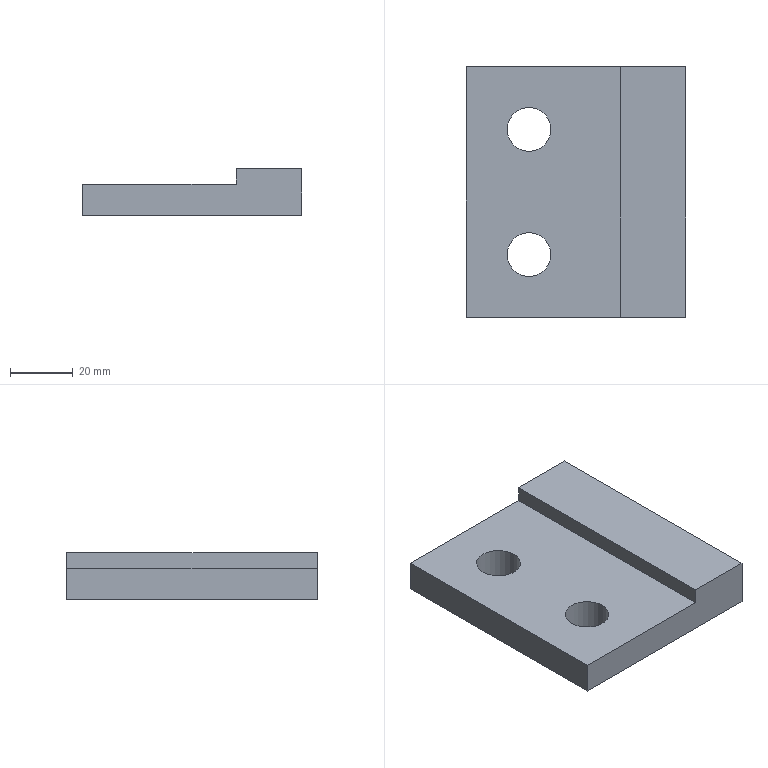Part | NX | features solid 2 | 1 solid | 10 faces | box 70 x 80 x 15 mm | volume 61270 mm3 | plane 8 | cylinder 2 | commonest cylinder face diameters 14 x2
STEP:
#1=CARTESIAN_POINT('',(18.,860.,-27.021));
#2=VERTEX_POINT('',#1);
#3=CARTESIAN_POINT('',(25.,860.,-27.021));
#4=DIRECTION('',(0.,0.,1.));
#5=DIRECTION('',(-1.,0.,0.));
#6=AXIS2_PLACEMENT_3D('',#3,#4,#5);
#7=CIRCLE('',#6,7.);
#8=EDGE_CURVE('',#2,#2,#7,.F.);
#9=ORIENTED_EDGE('',*,*,#8,.T.);
#10=EDGE_LOOP('',(#9));
#11=FACE_BOUND('',#10,.T.);
#12=CARTESIAN_POINT('',(54.128,880.,-27.021));
#13=VERTEX_POINT('',#12);
#14=CARTESIAN_POINT('',(54.128,800.,-27.021));
#15=VERTEX_POINT('',#14);
#16=CARTESIAN_POINT('',(54.128,890.,-27.021));
#17=DIRECTION('',(0.,-1.,0.));
#18=VECTOR('',#17,1000.);
#19=LINE('',#16,#18);
#20=EDGE_CURVE('',#13,#15,#19,.T.);
#21=ORIENTED_EDGE('',*,*,#20,.F.);
#22=CARTESIAN_POINT('',(5.,880.,-27.021));
#23=VERTEX_POINT('',#22);
#24=CARTESIAN_POINT('',(54.128,880.,-27.021));
#25=DIRECTION('',(1.,0.,0.));
#26=VECTOR('',#25,1000.);
#27=LINE('',#24,#26);
#28=EDGE_CURVE('',#13,#23,#27,.F.);
#29=ORIENTED_EDGE('',*,*,#28,.T.);
#30=CARTESIAN_POINT('',(5.,800.,-27.021));
#31=VERTEX_POINT('',#30);
#32=CARTESIAN_POINT('',(5.,890.,-27.021));
#33=DIRECTION('',(0.,1.,0.));
#34=VECTOR('',#33,1000.);
#35=LINE('',#32,#34);
#36=EDGE_CURVE('',#23,#31,#35,.F.);
#37=ORIENTED_EDGE('',*,*,#36,.T.);
#38=CARTESIAN_POINT('',(54.128,800.,-27.021));
#39=DIRECTION('',(-1.,0.,0.));
#40=VECTOR('',#39,1000.);
#41=LINE('',#38,#40);
#42=EDGE_CURVE('',#15,#31,#41,.T.);
#43=ORIENTED_EDGE('',*,*,#42,.F.);
#44=EDGE_LOOP('',(#21,#29,#37,#43));
#45=FACE_BOUND('',#44,.T.);
#46=CARTESIAN_POINT('',(18.,820.,-27.021));
#47=VERTEX_POINT('',#46);
#48=CARTESIAN_POINT('',(25.,820.,-27.021));
#49=DIRECTION('',(0.,0.,1.));
#50=DIRECTION('',(-1.,0.,0.));
#51=AXIS2_PLACEMENT_3D('',#48,#49,#50);
#52=CIRCLE('',#51,7.);
#53=EDGE_CURVE('',#47,#47,#52,.F.);
#54=ORIENTED_EDGE('',*,*,#53,.T.);
#55=EDGE_LOOP('',(#54));
#56=FACE_BOUND('',#55,.T.);
#57=CARTESIAN_POINT('',(54.128,890.,-27.021));
#58=DIRECTION('',(0.,0.,-1.));
#59=DIRECTION('',(-1.,0.,0.));
#60=AXIS2_PLACEMENT_3D('',#57,#58,#59);
#61=PLANE('',#60);
#62=ADVANCED_FACE('',(#11,#45,#56),#61,.F.);
#63=CARTESIAN_POINT('',(18.,860.,-37.021));
#64=VERTEX_POINT('',#63);
#65=CARTESIAN_POINT('',(25.,860.,-37.021));
#66=DIRECTION('',(0.,0.,1.));
#67=DIRECTION('',(-1.,0.,0.));
#68=AXIS2_PLACEMENT_3D('',#65,#66,#67);
#69=CIRCLE('',#68,7.);
#70=EDGE_CURVE('',#64,#64,#69,.F.);
#71=ORIENTED_EDGE('',*,*,#70,.F.);
#72=EDGE_LOOP('',(#71));
#73=FACE_BOUND('',#72,.T.);
#74=CARTESIAN_POINT('',(75.,800.,-37.021));
#75=VERTEX_POINT('',#74);
#76=CARTESIAN_POINT('',(5.,800.,-37.021));
#77=VERTEX_POINT('',#76);
#78=CARTESIAN_POINT('',(54.128,800.,-37.021));
#79=DIRECTION('',(-1.,0.,0.));
#80=VECTOR('',#79,1000.);
#81=LINE('',#78,#80);
#82=EDGE_CURVE('',#75,#77,#81,.T.);
#83=ORIENTED_EDGE('',*,*,#82,.T.);
#84=CARTESIAN_POINT('',(5.,880.,-37.021));
#85=VERTEX_POINT('',#84);
#86=CARTESIAN_POINT('',(5.,890.,-37.021));
#87=DIRECTION('',(0.,1.,0.));
#88=VECTOR('',#87,1000.);
#89=LINE('',#86,#88);
#90=EDGE_CURVE('',#85,#77,#89,.F.);
#91=ORIENTED_EDGE('',*,*,#90,.F.);
#92=CARTESIAN_POINT('',(75.,880.,-37.021));
#93=VERTEX_POINT('',#92);
#94=CARTESIAN_POINT('',(54.128,880.,-37.021));
#95=DIRECTION('',(1.,0.,0.));
#96=VECTOR('',#95,1000.);
#97=LINE('',#94,#96);
#98=EDGE_CURVE('',#93,#85,#97,.F.);
#99=ORIENTED_EDGE('',*,*,#98,.F.);
#100=CARTESIAN_POINT('',(75.,890.,-37.021));
#101=DIRECTION('',(0.,-1.,0.));
#102=VECTOR('',#101,1000.);
#103=LINE('',#100,#102);
#104=EDGE_CURVE('',#93,#75,#103,.T.);
#105=ORIENTED_EDGE('',*,*,#104,.T.);
#106=EDGE_LOOP('',(#83,#91,#99,#105));
#107=FACE_BOUND('',#106,.T.);
#108=CARTESIAN_POINT('',(18.,820.,-37.021));
#109=VERTEX_POINT('',#108);
#110=CARTESIAN_POINT('',(25.,820.,-37.021));
#111=DIRECTION('',(0.,0.,1.));
#112=DIRECTION('',(-1.,0.,0.));
#113=AXIS2_PLACEMENT_3D('',#110,#111,#112);
#114=CIRCLE('',#113,7.);
#115=EDGE_CURVE('',#109,#109,#114,.F.);
#116=ORIENTED_EDGE('',*,*,#115,.F.);
#117=EDGE_LOOP('',(#116));
#118=FACE_BOUND('',#117,.T.);
#119=CARTESIAN_POINT('',(54.128,890.,-37.021));
#120=DIRECTION('',(0.,0.,-1.));
#121=DIRECTION('',(-1.,0.,0.));
#122=AXIS2_PLACEMENT_3D('',#119,#120,#121);
#123=PLANE('',#122);
#124=ADVANCED_FACE('',(#73,#107,#118),#123,.T.);
#125=CARTESIAN_POINT('',(75.,800.,-22.021));
#126=VERTEX_POINT('',#125);
#127=CARTESIAN_POINT('',(54.128,800.,-22.021));
#128=VERTEX_POINT('',#127);
#129=CARTESIAN_POINT('',(74.128,800.,-22.021));
#130=DIRECTION('',(-1.,0.,0.));
#131=VECTOR('',#130,1000.);
#132=LINE('',#129,#131);
#133=EDGE_CURVE('',#126,#128,#132,.T.);
#134=ORIENTED_EDGE('',*,*,#133,.F.);
#135=CARTESIAN_POINT('',(75.,880.,-22.021));
#136=VERTEX_POINT('',#135);
#137=CARTESIAN_POINT('',(75.,890.,-22.021));
#138=DIRECTION('',(0.,-1.,0.));
#139=VECTOR('',#138,1000.);
#140=LINE('',#137,#139);
#141=EDGE_CURVE('',#136,#126,#140,.T.);
#142=ORIENTED_EDGE('',*,*,#141,.F.);
#143=CARTESIAN_POINT('',(54.128,880.,-22.021));
#144=VERTEX_POINT('',#143);
#145=CARTESIAN_POINT('',(54.128,880.,-22.021));
#146=DIRECTION('',(1.,0.,0.));
#147=VECTOR('',#146,1000.);
#148=LINE('',#145,#147);
#149=EDGE_CURVE('',#136,#144,#148,.F.);
#150=ORIENTED_EDGE('',*,*,#149,.T.);
#151=CARTESIAN_POINT('',(54.128,890.,-22.021));
#152=DIRECTION('',(0.,-1.,0.));
#153=VECTOR('',#152,1000.);
#154=LINE('',#151,#153);
#155=EDGE_CURVE('',#144,#128,#154,.T.);
#156=ORIENTED_EDGE('',*,*,#155,.T.);
#157=EDGE_LOOP('',(#134,#142,#150,#156));
#158=FACE_BOUND('',#157,.T.);
#159=CARTESIAN_POINT('',(74.128,890.,-22.021));
#160=DIRECTION('',(0.,0.,-1.));
#161=DIRECTION('',(0.,-1.,0.));
#162=AXIS2_PLACEMENT_3D('',#159,#160,#161);
#163=PLANE('',#162);
#164=ADVANCED_FACE('',(#158),#163,.F.);
#165=ORIENTED_EDGE('',*,*,#155,.F.);
#166=CARTESIAN_POINT('',(54.128,880.,-27.021));
#167=DIRECTION('',(0.,0.,-1.));
#168=VECTOR('',#167,1000.);
#169=LINE('',#166,#168);
#170=EDGE_CURVE('',#13,#144,#169,.F.);
#171=ORIENTED_EDGE('',*,*,#170,.F.);
#172=ORIENTED_EDGE('',*,*,#20,.T.);
#173=CARTESIAN_POINT('',(54.128,800.,-27.021));
#174=DIRECTION('',(0.,0.,1.));
#175=VECTOR('',#174,1000.);
#176=LINE('',#173,#175);
#177=EDGE_CURVE('',#15,#128,#176,.T.);
#178=ORIENTED_EDGE('',*,*,#177,.T.);
#179=EDGE_LOOP('',(#165,#171,#172,#178));
#180=FACE_BOUND('',#179,.T.);
#181=CARTESIAN_POINT('',(54.128,890.,-27.021));
#182=DIRECTION('',(1.,0.,0.));
#183=DIRECTION('',(0.,0.,-1.));
#184=AXIS2_PLACEMENT_3D('',#181,#182,#183);
#185=PLANE('',#184);
#186=ADVANCED_FACE('',(#180),#185,.F.);
#187=CARTESIAN_POINT('',(5.,880.,7.941));
#188=DIRECTION('',(0.,0.,1.));
#189=VECTOR('',#188,1000.);
#190=LINE('',#187,#189);
#191=EDGE_CURVE('',#85,#23,#190,.T.);
#192=ORIENTED_EDGE('',*,*,#191,.F.);
#193=ORIENTED_EDGE('',*,*,#90,.T.);
#194=CARTESIAN_POINT('',(5.,800.,-27.021));
#195=DIRECTION('',(0.,0.,-1.));
#196=VECTOR('',#195,1000.);
#197=LINE('',#194,#196);
#198=EDGE_CURVE('',#77,#31,#197,.F.);
#199=ORIENTED_EDGE('',*,*,#198,.T.);
#200=ORIENTED_EDGE('',*,*,#36,.F.);
#201=EDGE_LOOP('',(#192,#193,#199,#200));
#202=FACE_BOUND('',#201,.T.);
#203=CARTESIAN_POINT('',(5.,894.636,7.941));
#204=DIRECTION('',(-1.,0.,0.));
#205=DIRECTION('',(0.,0.,-1.));
#206=AXIS2_PLACEMENT_3D('',#203,#204,#205);
#207=PLANE('',#206);
#208=ADVANCED_FACE('',(#202),#207,.T.);
#209=CARTESIAN_POINT('',(75.,880.,-27.021));
#210=DIRECTION('',(0.,0.,-1.));
#211=VECTOR('',#210,1000.);
#212=LINE('',#209,#211);
#213=EDGE_CURVE('',#93,#136,#212,.F.);
#214=ORIENTED_EDGE('',*,*,#213,.F.);
#215=ORIENTED_EDGE('',*,*,#98,.T.);
#216=ORIENTED_EDGE('',*,*,#191,.T.);
#217=ORIENTED_EDGE('',*,*,#28,.F.);
#218=ORIENTED_EDGE('',*,*,#170,.T.);
#219=ORIENTED_EDGE('',*,*,#149,.F.);
#220=EDGE_LOOP('',(#214,#215,#216,#217,#218,#219));
#221=FACE_BOUND('',#220,.T.);
#222=CARTESIAN_POINT('',(54.128,880.,-27.021));
#223=DIRECTION('',(0.,1.,0.));
#224=DIRECTION('',(-1.,0.,0.));
#225=AXIS2_PLACEMENT_3D('',#222,#223,#224);
#226=PLANE('',#225);
#227=ADVANCED_FACE('',(#221),#226,.T.);
#228=ORIENTED_EDGE('',*,*,#104,.F.);
#229=ORIENTED_EDGE('',*,*,#213,.T.);
#230=ORIENTED_EDGE('',*,*,#141,.T.);
#231=CARTESIAN_POINT('',(75.,800.,-27.021));
#232=DIRECTION('',(0.,0.,1.));
#233=VECTOR('',#232,1000.);
#234=LINE('',#231,#233);
#235=EDGE_CURVE('',#75,#126,#234,.T.);
#236=ORIENTED_EDGE('',*,*,#235,.F.);
#237=EDGE_LOOP('',(#228,#229,#230,#236));
#238=FACE_BOUND('',#237,.T.);
#239=CARTESIAN_POINT('',(75.,890.,-27.021));
#240=DIRECTION('',(-1.,0.,0.));
#241=DIRECTION('',(0.,-1.,0.));
#242=AXIS2_PLACEMENT_3D('',#239,#240,#241);
#243=PLANE('',#242);
#244=ADVANCED_FACE('',(#238),#243,.F.);
#245=ORIENTED_EDGE('',*,*,#198,.F.);
#246=ORIENTED_EDGE('',*,*,#82,.F.);
#247=ORIENTED_EDGE('',*,*,#235,.T.);
#248=ORIENTED_EDGE('',*,*,#133,.T.);
#249=ORIENTED_EDGE('',*,*,#177,.F.);
#250=ORIENTED_EDGE('',*,*,#42,.T.);
#251=EDGE_LOOP('',(#245,#246,#247,#248,#249,#250));
#252=FACE_BOUND('',#251,.T.);
#253=CARTESIAN_POINT('',(54.128,800.,-27.021));
#254=DIRECTION('',(0.,1.,0.));
#255=DIRECTION('',(-1.,0.,0.));
#256=AXIS2_PLACEMENT_3D('',#253,#254,#255);
#257=PLANE('',#256);
#258=ADVANCED_FACE('',(#252),#257,.F.);
#259=ORIENTED_EDGE('',*,*,#70,.T.);
#260=EDGE_LOOP('',(#259));
#261=FACE_BOUND('',#260,.T.);
#262=ORIENTED_EDGE('',*,*,#8,.F.);
#263=EDGE_LOOP('',(#262));
#264=FACE_BOUND('',#263,.T.);
#265=CARTESIAN_POINT('',(25.,860.,-72.021));
#266=DIRECTION('',(0.,0.,1.));
#267=DIRECTION('',(1.,0.,0.));
#268=AXIS2_PLACEMENT_3D('',#265,#266,#267);
#269=CYLINDRICAL_SURFACE('',#268,7.);
#270=ADVANCED_FACE('',(#261,#264),#269,.F.);
#271=ORIENTED_EDGE('',*,*,#115,.T.);
#272=EDGE_LOOP('',(#271));
#273=FACE_BOUND('',#272,.T.);
#274=ORIENTED_EDGE('',*,*,#53,.F.);
#275=EDGE_LOOP('',(#274));
#276=FACE_BOUND('',#275,.T.);
#277=CARTESIAN_POINT('',(25.,820.,-72.021));
#278=DIRECTION('',(0.,0.,1.));
#279=DIRECTION('',(1.,0.,0.));
#280=AXIS2_PLACEMENT_3D('',#277,#278,#279);
#281=CYLINDRICAL_SURFACE('',#280,7.);
#282=ADVANCED_FACE('',(#273,#276),#281,.F.);
#283=CLOSED_SHELL('',(#62,#124,#164,#186,#208,#227,#244,#258,#270,#282));
#284=MANIFOLD_SOLID_BREP('',#283);
#285=(LENGTH_UNIT()NAMED_UNIT(*)SI_UNIT(.MILLI.,.METRE.));
#286=UNCERTAINTY_MEASURE_WITH_UNIT(LENGTH_MEASURE(0.00001),#285,'','');
#287=(NAMED_UNIT(*)PLANE_ANGLE_UNIT()SI_UNIT($,.RADIAN.));
#288=(NAMED_UNIT(*)SI_UNIT($,.STERADIAN.)SOLID_ANGLE_UNIT());
#289=(GEOMETRIC_REPRESENTATION_CONTEXT(3)GLOBAL_UNCERTAINTY_ASSIGNED_CONTEXT((#286))GLOBAL_UNIT_ASSIGNED_CONTEXT((#285,#287,#288))REPRESENTATION_CONTEXT('',''));
#290=ADVANCED_BREP_SHAPE_REPRESENTATION('',(#284),#289);